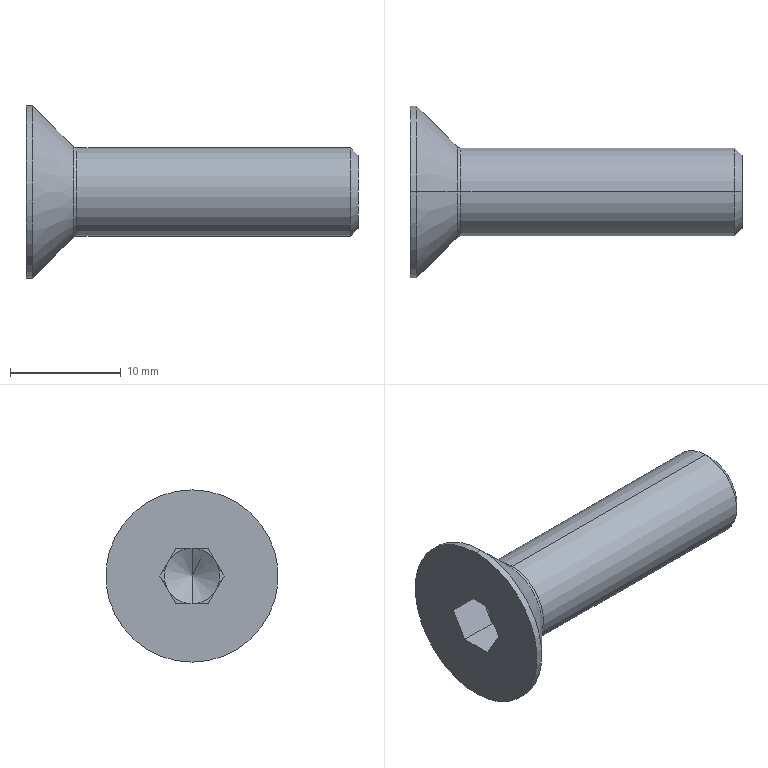Part | STEP file | socket countersunk head screw_din_DIN 7991 - M8 x 30 --- 21.8N | 1 solid | 26 faces | box 30 x 15.57 x 15.57 mm | volume 1740 mm3 | plane 14 | cone 6 | cylinder 4 | torus 2 | commonest cylinder face diameters 8 x2 15.57 x2